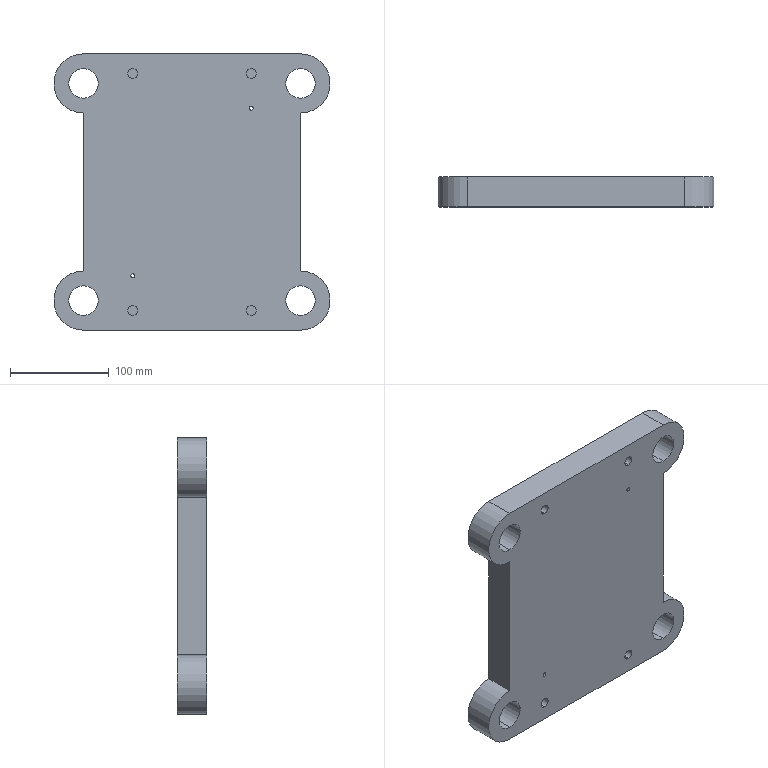Part | SolidWorks | features ICE 4, Extrusion 1, Fillet 1, HoleWzd 1, MirrorPattern 1 | 1 solid | 51 faces | box 280 x 30 x 280 mm | volume 1868516 mm3 | cylinder 34 | plane 15 | torus 2 | commonest cylinder face diameters 10 x8 12 x8 30 x8 4 x4 60 x4 80 x2
STEP:
#1=CARTESIAN_POINT('',(0.,5.,-31.));
#2=VERTEX_POINT('',#1);
#3=CARTESIAN_POINT('',(0.,5.,-19.));
#4=VERTEX_POINT('',#3);
#5=CARTESIAN_POINT('',(0.,5.,-25.));
#6=DIRECTION('',(0.,1.,0.));
#7=DIRECTION('',(0.,0.,1.));
#8=AXIS2_PLACEMENT_3D('',#5,#6,#7);
#9=CIRCLE('',#8,6.);
#10=EDGE_CURVE('',#2,#4,#9,.T.);
#11=ORIENTED_EDGE('',*,*,#10,.F.);
#12=CARTESIAN_POINT('',(0.,20.,-31.));
#13=VERTEX_POINT('',#12);
#14=CARTESIAN_POINT('',(0.,5.,-31.));
#15=DIRECTION('',(0.,1.,0.));
#16=VECTOR('',#15,1000.);
#17=LINE('',#14,#16);
#18=EDGE_CURVE('',#2,#13,#17,.T.);
#19=ORIENTED_EDGE('',*,*,#18,.T.);
#20=CARTESIAN_POINT('',(0.,20.,-19.));
#21=VERTEX_POINT('',#20);
#22=CARTESIAN_POINT('',(0.,20.,-25.));
#23=DIRECTION('',(0.,1.,0.));
#24=DIRECTION('',(0.,0.,1.));
#25=AXIS2_PLACEMENT_3D('',#22,#23,#24);
#26=CIRCLE('',#25,6.);
#27=EDGE_CURVE('',#13,#21,#26,.T.);
#28=ORIENTED_EDGE('',*,*,#27,.T.);
#29=CARTESIAN_POINT('',(0.,5.,-19.));
#30=DIRECTION('',(0.,1.,0.));
#31=VECTOR('',#30,1000.);
#32=LINE('',#29,#31);
#33=EDGE_CURVE('',#4,#21,#32,.T.);
#34=ORIENTED_EDGE('',*,*,#33,.F.);
#35=EDGE_LOOP('',(#11,#19,#28,#34));
#36=FACE_OUTER_BOUND('',#35,.T.);
#37=CARTESIAN_POINT('',(0.,5.,-25.));
#38=DIRECTION('',(0.,1.,0.));
#39=DIRECTION('',(0.,0.,1.));
#40=AXIS2_PLACEMENT_3D('',#37,#38,#39);
#41=CYLINDRICAL_SURFACE('',#40,6.);
#42=ADVANCED_FACE('',(#36),#41,.F.);
#43=CARTESIAN_POINT('',(-25.4,5.,-6.));
#44=VERTEX_POINT('',#43);
#45=CARTESIAN_POINT('',(-25.4,5.,6.));
#46=VERTEX_POINT('',#45);
#47=CARTESIAN_POINT('',(-25.4,5.,0.));
#48=DIRECTION('',(0.,1.,0.));
#49=DIRECTION('',(0.,0.,1.));
#50=AXIS2_PLACEMENT_3D('',#47,#48,#49);
#51=CIRCLE('',#50,6.);
#52=EDGE_CURVE('',#44,#46,#51,.T.);
#53=ORIENTED_EDGE('',*,*,#52,.F.);
#54=CARTESIAN_POINT('',(-25.4,20.,-6.));
#55=VERTEX_POINT('',#54);
#56=CARTESIAN_POINT('',(-25.4,5.,-6.));
#57=DIRECTION('',(0.,1.,0.));
#58=VECTOR('',#57,1000.);
#59=LINE('',#56,#58);
#60=EDGE_CURVE('',#44,#55,#59,.T.);
#61=ORIENTED_EDGE('',*,*,#60,.T.);
#62=CARTESIAN_POINT('',(-25.4,20.,6.));
#63=VERTEX_POINT('',#62);
#64=CARTESIAN_POINT('',(-25.4,20.,0.));
#65=DIRECTION('',(0.,1.,0.));
#66=DIRECTION('',(0.,0.,1.));
#67=AXIS2_PLACEMENT_3D('',#64,#65,#66);
#68=CIRCLE('',#67,6.);
#69=EDGE_CURVE('',#55,#63,#68,.T.);
#70=ORIENTED_EDGE('',*,*,#69,.T.);
#71=CARTESIAN_POINT('',(-25.4,5.,6.));
#72=DIRECTION('',(0.,1.,0.));
#73=VECTOR('',#72,1000.);
#74=LINE('',#71,#73);
#75=EDGE_CURVE('',#46,#63,#74,.T.);
#76=ORIENTED_EDGE('',*,*,#75,.F.);
#77=EDGE_LOOP('',(#53,#61,#70,#76));
#78=FACE_OUTER_BOUND('',#77,.T.);
#79=CARTESIAN_POINT('',(-25.4,5.,0.));
#80=DIRECTION('',(0.,1.,0.));
#81=DIRECTION('',(0.,0.,1.));
#82=AXIS2_PLACEMENT_3D('',#79,#80,#81);
#83=CYLINDRICAL_SURFACE('',#82,6.);
#84=ADVANCED_FACE('',(#78),#83,.F.);
#85=CARTESIAN_POINT('',(0.,5.,19.));
#86=VERTEX_POINT('',#85);
#87=CARTESIAN_POINT('',(0.,5.,31.));
#88=VERTEX_POINT('',#87);
#89=CARTESIAN_POINT('',(0.,5.,25.));
#90=DIRECTION('',(0.,1.,0.));
#91=DIRECTION('',(0.,0.,1.));
#92=AXIS2_PLACEMENT_3D('',#89,#90,#91);
#93=CIRCLE('',#92,6.);
#94=EDGE_CURVE('',#86,#88,#93,.T.);
#95=ORIENTED_EDGE('',*,*,#94,.F.);
#96=CARTESIAN_POINT('',(0.,20.,19.));
#97=VERTEX_POINT('',#96);
#98=CARTESIAN_POINT('',(0.,5.,19.));
#99=DIRECTION('',(0.,1.,0.));
#100=VECTOR('',#99,1000.);
#101=LINE('',#98,#100);
#102=EDGE_CURVE('',#86,#97,#101,.T.);
#103=ORIENTED_EDGE('',*,*,#102,.T.);
#104=CARTESIAN_POINT('',(0.,20.,31.));
#105=VERTEX_POINT('',#104);
#106=CARTESIAN_POINT('',(0.,20.,25.));
#107=DIRECTION('',(0.,1.,0.));
#108=DIRECTION('',(0.,0.,1.));
#109=AXIS2_PLACEMENT_3D('',#106,#107,#108);
#110=CIRCLE('',#109,6.);
#111=EDGE_CURVE('',#97,#105,#110,.T.);
#112=ORIENTED_EDGE('',*,*,#111,.T.);
#113=CARTESIAN_POINT('',(0.,5.,31.));
#114=DIRECTION('',(0.,1.,0.));
#115=VECTOR('',#114,1000.);
#116=LINE('',#113,#115);
#117=EDGE_CURVE('',#88,#105,#116,.T.);
#118=ORIENTED_EDGE('',*,*,#117,.F.);
#119=EDGE_LOOP('',(#95,#103,#112,#118));
#120=FACE_OUTER_BOUND('',#119,.T.);
#121=CARTESIAN_POINT('',(0.,5.,25.));
#122=DIRECTION('',(0.,1.,0.));
#123=DIRECTION('',(0.,0.,1.));
#124=AXIS2_PLACEMENT_3D('',#121,#122,#123);
#125=CYLINDRICAL_SURFACE('',#124,6.);
#126=ADVANCED_FACE('',(#120),#125,.F.);
#127=CARTESIAN_POINT('',(25.,5.,-6.));
#128=VERTEX_POINT('',#127);
#129=CARTESIAN_POINT('',(25.,5.,6.));
#130=VERTEX_POINT('',#129);
#131=CARTESIAN_POINT('',(25.,5.,0.));
#132=DIRECTION('',(0.,1.,0.));
#133=DIRECTION('',(0.,0.,1.));
#134=AXIS2_PLACEMENT_3D('',#131,#132,#133);
#135=CIRCLE('',#134,6.);
#136=EDGE_CURVE('',#128,#130,#135,.T.);
#137=ORIENTED_EDGE('',*,*,#136,.F.);
#138=CARTESIAN_POINT('',(25.,20.,-6.));
#139=VERTEX_POINT('',#138);
#140=CARTESIAN_POINT('',(25.,5.,-6.));
#141=DIRECTION('',(0.,1.,0.));
#142=VECTOR('',#141,1000.);
#143=LINE('',#140,#142);
#144=EDGE_CURVE('',#128,#139,#143,.T.);
#145=ORIENTED_EDGE('',*,*,#144,.T.);
#146=CARTESIAN_POINT('',(25.,20.,6.));
#147=VERTEX_POINT('',#146);
#148=CARTESIAN_POINT('',(25.,20.,0.));
#149=DIRECTION('',(0.,1.,0.));
#150=DIRECTION('',(0.,0.,1.));
#151=AXIS2_PLACEMENT_3D('',#148,#149,#150);
#152=CIRCLE('',#151,6.);
#153=EDGE_CURVE('',#139,#147,#152,.T.);
#154=ORIENTED_EDGE('',*,*,#153,.T.);
#155=CARTESIAN_POINT('',(25.,5.,6.));
#156=DIRECTION('',(0.,1.,0.));
#157=VECTOR('',#156,1000.);
#158=LINE('',#155,#157);
#159=EDGE_CURVE('',#130,#147,#158,.T.);
#160=ORIENTED_EDGE('',*,*,#159,.F.);
#161=EDGE_LOOP('',(#137,#145,#154,#160));
#162=FACE_OUTER_BOUND('',#161,.T.);
#163=CARTESIAN_POINT('',(25.,5.,0.));
#164=DIRECTION('',(0.,1.,0.));
#165=DIRECTION('',(0.,0.,1.));
#166=AXIS2_PLACEMENT_3D('',#163,#164,#165);
#167=CYLINDRICAL_SURFACE('',#166,6.);
#168=ADVANCED_FACE('',(#162),#167,.F.);
#169=CARTESIAN_POINT('',(0.,30.,-42.));
#170=VERTEX_POINT('',#169);
#171=CARTESIAN_POINT('',(0.,30.,42.));
#172=VERTEX_POINT('',#171);
#173=CARTESIAN_POINT('',(0.,30.,0.));
#174=DIRECTION('',(0.,-1.,0.));
#175=DIRECTION('',(0.,0.,1.));
#176=AXIS2_PLACEMENT_3D('',#173,#174,#175);
#177=CIRCLE('',#176,42.);
#178=EDGE_CURVE('',#170,#172,#177,.T.);
#179=ORIENTED_EDGE('',*,*,#178,.F.);
#180=CARTESIAN_POINT('',(0.,28.,-40.));
#181=VERTEX_POINT('',#180);
#182=CARTESIAN_POINT('',(0.,28.,-42.));
#183=DIRECTION('',(1.,0.,0.));
#184=DIRECTION('',(0.,0.,-1.));
#185=AXIS2_PLACEMENT_3D('',#182,#183,#184);
#186=CIRCLE('',#185,2.);
#187=EDGE_CURVE('',#170,#181,#186,.T.);
#188=ORIENTED_EDGE('',*,*,#187,.T.);
#189=CARTESIAN_POINT('',(0.,28.,40.));
#190=VERTEX_POINT('',#189);
#191=CARTESIAN_POINT('',(0.,28.,0.));
#192=DIRECTION('',(0.,1.,0.));
#193=DIRECTION('',(0.,0.,1.));
#194=AXIS2_PLACEMENT_3D('',#191,#192,#193);
#195=CIRCLE('',#194,40.);
#196=EDGE_CURVE('',#190,#181,#195,.T.);
#197=ORIENTED_EDGE('',*,*,#196,.F.);
#198=CARTESIAN_POINT('',(0.,28.,42.));
#199=DIRECTION('',(-1.,0.,0.));
#200=DIRECTION('',(0.,0.,1.));
#201=AXIS2_PLACEMENT_3D('',#198,#199,#200);
#202=CIRCLE('',#201,2.);
#203=EDGE_CURVE('',#172,#190,#202,.T.);
#204=ORIENTED_EDGE('',*,*,#203,.F.);
#205=EDGE_LOOP('',(#179,#188,#197,#204));
#206=FACE_OUTER_BOUND('',#205,.T.);
#207=CARTESIAN_POINT('',(0.,28.,0.));
#208=DIRECTION('',(0.,1.,0.));
#209=DIRECTION('',(0.,0.,1.));
#210=AXIS2_PLACEMENT_3D('',#207,#208,#209);
#211=TOROIDAL_SURFACE('',#210,42.,2.);
#212=ADVANCED_FACE('',(#206),#211,.T.);
#213=CARTESIAN_POINT('',(0.,20.,-40.));
#214=VERTEX_POINT('',#213);
#215=CARTESIAN_POINT('',(0.,20.,40.));
#216=VERTEX_POINT('',#215);
#217=CARTESIAN_POINT('',(0.,20.,0.));
#218=DIRECTION('',(0.,1.,0.));
#219=DIRECTION('',(0.,0.,1.));
#220=AXIS2_PLACEMENT_3D('',#217,#218,#219);
#221=CIRCLE('',#220,40.);
#222=EDGE_CURVE('',#214,#216,#221,.T.);
#223=ORIENTED_EDGE('',*,*,#222,.F.);
#224=CARTESIAN_POINT('',(0.,20.,-40.));
#225=DIRECTION('',(0.,1.,0.));
#226=VECTOR('',#225,1000.);
#227=LINE('',#224,#226);
#228=EDGE_CURVE('',#214,#181,#227,.T.);
#229=ORIENTED_EDGE('',*,*,#228,.T.);
#230=CARTESIAN_POINT('',(0.,28.,0.));
#231=DIRECTION('',(0.,1.,0.));
#232=DIRECTION('',(0.,0.,1.));
#233=AXIS2_PLACEMENT_3D('',#230,#231,#232);
#234=CIRCLE('',#233,40.);
#235=EDGE_CURVE('',#181,#190,#234,.T.);
#236=ORIENTED_EDGE('',*,*,#235,.T.);
#237=CARTESIAN_POINT('',(0.,20.,40.));
#238=DIRECTION('',(0.,1.,0.));
#239=VECTOR('',#238,1000.);
#240=LINE('',#237,#239);
#241=EDGE_CURVE('',#216,#190,#240,.T.);
#242=ORIENTED_EDGE('',*,*,#241,.F.);
#243=EDGE_LOOP('',(#223,#229,#236,#242));
#244=FACE_OUTER_BOUND('',#243,.T.);
#245=CARTESIAN_POINT('',(0.,20.,0.));
#246=DIRECTION('',(0.,1.,0.));
#247=DIRECTION('',(0.,0.,1.));
#248=AXIS2_PLACEMENT_3D('',#245,#246,#247);
#249=CYLINDRICAL_SURFACE('',#248,40.);
#250=ADVANCED_FACE('',(#244),#249,.F.);
#251=CARTESIAN_POINT('',(-60.,20.,-115.));
#252=VERTEX_POINT('',#251);
#253=CARTESIAN_POINT('',(-60.,20.,-125.));
#254=VERTEX_POINT('',#253);
#255=CARTESIAN_POINT('',(-60.,20.,-120.));
#256=DIRECTION('',(0.,-1.,0.));
#257=DIRECTION('',(0.,0.,1.));
#258=AXIS2_PLACEMENT_3D('',#255,#256,#257);
#259=CIRCLE('',#258,5.);
#260=EDGE_CURVE('',#252,#254,#259,.T.);
#261=ORIENTED_EDGE('',*,*,#260,.F.);
#262=CARTESIAN_POINT('',(-60.,0.,-115.));
#263=VERTEX_POINT('',#262);
#264=CARTESIAN_POINT('',(-60.,20.,-115.));
#265=DIRECTION('',(0.,-1.,0.));
#266=VECTOR('',#265,1000.);
#267=LINE('',#264,#266);
#268=EDGE_CURVE('',#252,#263,#267,.T.);
#269=ORIENTED_EDGE('',*,*,#268,.T.);
#270=CARTESIAN_POINT('',(-60.,0.,-125.));
#271=VERTEX_POINT('',#270);
#272=CARTESIAN_POINT('',(-60.,0.,-120.));
#273=DIRECTION('',(0.,-1.,0.));
#274=DIRECTION('',(0.,0.,1.));
#275=AXIS2_PLACEMENT_3D('',#272,#273,#274);
#276=CIRCLE('',#275,5.);
#277=EDGE_CURVE('',#263,#271,#276,.T.);
#278=ORIENTED_EDGE('',*,*,#277,.T.);
#279=CARTESIAN_POINT('',(-60.,20.,-125.));
#280=DIRECTION('',(0.,-1.,0.));
#281=VECTOR('',#280,1000.);
#282=LINE('',#279,#281);
#283=EDGE_CURVE('',#254,#271,#282,.T.);
#284=ORIENTED_EDGE('',*,*,#283,.F.);
#285=EDGE_LOOP('',(#261,#269,#278,#284));
#286=FACE_OUTER_BOUND('',#285,.T.);
#287=CARTESIAN_POINT('',(-60.,20.,-120.));
#288=DIRECTION('',(0.,-1.,0.));
#289=DIRECTION('',(0.,0.,-1.));
#290=AXIS2_PLACEMENT_3D('',#287,#288,#289);
#291=CYLINDRICAL_SURFACE('',#290,5.);
#292=ADVANCED_FACE('',(#286),#291,.F.);
#293=CARTESIAN_POINT('',(60.,20.,-115.));
#294=VERTEX_POINT('',#293);
#295=CARTESIAN_POINT('',(60.,20.,-125.));
#296=VERTEX_POINT('',#295);
#297=CARTESIAN_POINT('',(60.,20.,-120.));
#298=DIRECTION('',(0.,-1.,0.));
#299=DIRECTION('',(0.,0.,-1.));
#300=AXIS2_PLACEMENT_3D('',#297,#298,#299);
#301=CIRCLE('',#300,5.);
#302=EDGE_CURVE('',#294,#296,#301,.T.);
#303=ORIENTED_EDGE('',*,*,#302,.F.);
#304=CARTESIAN_POINT('',(60.,0.,-115.));
#305=VERTEX_POINT('',#304);
#306=CARTESIAN_POINT('',(60.,20.,-115.));
#307=DIRECTION('',(0.,-1.,0.));
#308=VECTOR('',#307,1000.);
#309=LINE('',#306,#308);
#310=EDGE_CURVE('',#294,#305,#309,.T.);
#311=ORIENTED_EDGE('',*,*,#310,.T.);
#312=CARTESIAN_POINT('',(60.,0.,-125.));
#313=VERTEX_POINT('',#312);
#314=CARTESIAN_POINT('',(60.,0.,-120.));
#315=DIRECTION('',(0.,-1.,0.));
#316=DIRECTION('',(0.,0.,-1.));
#317=AXIS2_PLACEMENT_3D('',#314,#315,#316);
#318=CIRCLE('',#317,5.);
#319=EDGE_CURVE('',#305,#313,#318,.T.);
#320=ORIENTED_EDGE('',*,*,#319,.T.);
#321=CARTESIAN_POINT('',(60.,20.,-125.));
#322=DIRECTION('',(0.,-1.,0.));
#323=VECTOR('',#322,1000.);
#324=LINE('',#321,#323);
#325=EDGE_CURVE('',#296,#313,#324,.T.);
#326=ORIENTED_EDGE('',*,*,#325,.F.);
#327=EDGE_LOOP('',(#303,#311,#320,#326));
#328=FACE_OUTER_BOUND('',#327,.T.);
#329=CARTESIAN_POINT('',(60.,20.,-120.));
#330=DIRECTION('',(0.,-1.,0.));
#331=DIRECTION('',(0.,0.,-1.));
#332=AXIS2_PLACEMENT_3D('',#329,#330,#331);
#333=CYLINDRICAL_SURFACE('',#332,5.);
#334=ADVANCED_FACE('',(#328),#333,.F.);
#335=CARTESIAN_POINT('',(60.,20.,125.));
#336=VERTEX_POINT('',#335);
#337=CARTESIAN_POINT('',(60.,20.,115.));
#338=VERTEX_POINT('',#337);
#339=CARTESIAN_POINT('',(60.,20.,120.));
#340=DIRECTION('',(0.,-1.,0.));
#341=DIRECTION('',(0.,0.,1.));
#342=AXIS2_PLACEMENT_3D('',#339,#340,#341);
#343=CIRCLE('',#342,5.);
#344=EDGE_CURVE('',#336,#338,#343,.T.);
#345=ORIENTED_EDGE('',*,*,#344,.F.);
#346=CARTESIAN_POINT('',(60.,0.,125.));
#347=VERTEX_POINT('',#346);
#348=CARTESIAN_POINT('',(60.,20.,125.));
#349=DIRECTION('',(0.,-1.,0.));
#350=VECTOR('',#349,1000.);
#351=LINE('',#348,#350);
#352=EDGE_CURVE('',#336,#347,#351,.T.);
#353=ORIENTED_EDGE('',*,*,#352,.T.);
#354=CARTESIAN_POINT('',(60.,0.,115.));
#355=VERTEX_POINT('',#354);
#356=CARTESIAN_POINT('',(60.,0.,120.));
#357=DIRECTION('',(0.,-1.,0.));
#358=DIRECTION('',(0.,0.,1.));
#359=AXIS2_PLACEMENT_3D('',#356,#357,#358);
#360=CIRCLE('',#359,5.);
#361=EDGE_CURVE('',#347,#355,#360,.T.);
#362=ORIENTED_EDGE('',*,*,#361,.T.);
#363=CARTESIAN_POINT('',(60.,20.,115.));
#364=DIRECTION('',(0.,-1.,0.));
#365=VECTOR('',#364,1000.);
#366=LINE('',#363,#365);
#367=EDGE_CURVE('',#338,#355,#366,.T.);
#368=ORIENTED_EDGE('',*,*,#367,.F.);
#369=EDGE_LOOP('',(#345,#353,#362,#368));
#370=FACE_OUTER_BOUND('',#369,.T.);
#371=CARTESIAN_POINT('',(60.,20.,120.));
#372=DIRECTION('',(0.,-1.,0.));
#373=DIRECTION('',(0.,0.,-1.));
#374=AXIS2_PLACEMENT_3D('',#371,#372,#373);
#375=CYLINDRICAL_SURFACE('',#374,5.);
#376=ADVANCED_FACE('',(#370),#375,.F.);
#377=CARTESIAN_POINT('',(-60.,20.,125.));
#378=VERTEX_POINT('',#377);
#379=CARTESIAN_POINT('',(-60.,20.,115.));
#380=VERTEX_POINT('',#379);
#381=CARTESIAN_POINT('',(-60.,20.,120.));
#382=DIRECTION('',(0.,-1.,0.));
#383=DIRECTION('',(0.,0.,-1.));
#384=AXIS2_PLACEMENT_3D('',#381,#382,#383);
#385=CIRCLE('',#384,5.);
#386=EDGE_CURVE('',#378,#380,#385,.T.);
#387=ORIENTED_EDGE('',*,*,#386,.F.);
#388=CARTESIAN_POINT('',(-60.,0.,125.));
#389=VERTEX_POINT('',#388);
#390=CARTESIAN_POINT('',(-60.,20.,125.));
#391=DIRECTION('',(0.,-1.,0.));
#392=VECTOR('',#391,1000.);
#393=LINE('',#390,#392);
#394=EDGE_CURVE('',#378,#389,#393,.T.);
#395=ORIENTED_EDGE('',*,*,#394,.T.);
#396=CARTESIAN_POINT('',(-60.,0.,115.));
#397=VERTEX_POINT('',#396);
#398=CARTESIAN_POINT('',(-60.,0.,120.));
#399=DIRECTION('',(0.,-1.,0.));
#400=DIRECTION('',(0.,0.,-1.));
#401=AXIS2_PLACEMENT_3D('',#398,#399,#400);
#402=CIRCLE('',#401,5.);
#403=EDGE_CURVE('',#389,#397,#402,.T.);
#404=ORIENTED_EDGE('',*,*,#403,.T.);
#405=CARTESIAN_POINT('',(-60.,20.,115.));
#406=DIRECTION('',(0.,-1.,0.));
#407=VECTOR('',#406,1000.);
#408=LINE('',#405,#407);
#409=EDGE_CURVE('',#380,#397,#408,.T.);
#410=ORIENTED_EDGE('',*,*,#409,.F.);
#411=EDGE_LOOP('',(#387,#395,#404,#410));
#412=FACE_OUTER_BOUND('',#411,.T.);
#413=CARTESIAN_POINT('',(-60.,20.,120.));
#414=DIRECTION('',(0.,-1.,0.));
#415=DIRECTION('',(0.,0.,-1.));
#416=AXIS2_PLACEMENT_3D('',#413,#414,#415);
#417=CYLINDRICAL_SURFACE('',#416,5.);
#418=ADVANCED_FACE('',(#412),#417,.F.);
#419=CARTESIAN_POINT('',(-60.,0.,-87.));
#420=VERTEX_POINT('',#419);
#421=CARTESIAN_POINT('',(-60.,0.,-83.));
#422=VERTEX_POINT('',#421);
#423=CARTESIAN_POINT('',(-60.,0.,-85.));
#424=DIRECTION('',(0.,1.,0.));
#425=DIRECTION('',(0.,0.,1.));
#426=AXIS2_PLACEMENT_3D('',#423,#424,#425);
#427=CIRCLE('',#426,2.);
#428=EDGE_CURVE('',#420,#422,#427,.T.);
#429=ORIENTED_EDGE('',*,*,#428,.F.);
#430=CARTESIAN_POINT('',(-60.,30.,-87.));
#431=VERTEX_POINT('',#430);
#432=CARTESIAN_POINT('',(-60.,0.,-87.));
#433=DIRECTION('',(0.,1.,0.));
#434=VECTOR('',#433,1000.);
#435=LINE('',#432,#434);
#436=EDGE_CURVE('',#420,#431,#435,.T.);
#437=ORIENTED_EDGE('',*,*,#436,.T.);
#438=CARTESIAN_POINT('',(-60.,30.,-83.));
#439=VERTEX_POINT('',#438);
#440=CARTESIAN_POINT('',(-60.,30.,-85.));
#441=DIRECTION('',(0.,1.,0.));
#442=DIRECTION('',(0.,0.,1.));
#443=AXIS2_PLACEMENT_3D('',#440,#441,#442);
#444=CIRCLE('',#443,2.);
#445=EDGE_CURVE('',#431,#439,#444,.T.);
#446=ORIENTED_EDGE('',*,*,#445,.T.);
#447=CARTESIAN_POINT('',(-60.,0.,-83.));
#448=DIRECTION('',(0.,1.,0.));
#449=VECTOR('',#448,1000.);
#450=LINE('',#447,#449);
#451=EDGE_CURVE('',#422,#439,#450,.T.);
#452=ORIENTED_EDGE('',*,*,#451,.F.);
#453=EDGE_LOOP('',(#429,#437,#446,#452));
#454=FACE_OUTER_BOUND('',#453,.T.);
#455=CARTESIAN_POINT('',(-60.,0.,-85.));
#456=DIRECTION('',(0.,1.,0.));
#457=DIRECTION('',(0.,0.,1.));
#458=AXIS2_PLACEMENT_3D('',#455,#456,#457);
#459=CYLINDRICAL_SURFACE('',#458,2.);
#460=ADVANCED_FACE('',(#454),#459,.F.);
#461=CARTESIAN_POINT('',(60.,0.,83.));
#462=VERTEX_POINT('',#461);
#463=CARTESIAN_POINT('',(60.,0.,87.));
#464=VERTEX_POINT('',#463);
#465=CARTESIAN_POINT('',(60.,0.,85.));
#466=DIRECTION('',(0.,1.,0.));
#467=DIRECTION('',(0.,0.,1.));
#468=AXIS2_PLACEMENT_3D('',#465,#466,#467);
#469=CIRCLE('',#468,2.);
#470=EDGE_CURVE('',#462,#464,#469,.T.);
#471=ORIENTED_EDGE('',*,*,#470,.F.);
#472=CARTESIAN_POINT('',(60.,30.,83.));
#473=VERTEX_POINT('',#472);
#474=CARTESIAN_POINT('',(60.,0.,83.));
#475=DIRECTION('',(0.,1.,0.));
#476=VECTOR('',#475,1000.);
#477=LINE('',#474,#476);
#478=EDGE_CURVE('',#462,#473,#477,.T.);
#479=ORIENTED_EDGE('',*,*,#478,.T.);
#480=CARTESIAN_POINT('',(60.,30.,87.));
#481=VERTEX_POINT('',#480);
#482=CARTESIAN_POINT('',(60.,30.,85.));
#483=DIRECTION('',(0.,1.,0.));
#484=DIRECTION('',(0.,0.,1.));
#485=AXIS2_PLACEMENT_3D('',#482,#483,#484);
#486=CIRCLE('',#485,2.);
#487=EDGE_CURVE('',#473,#481,#486,.T.);
#488=ORIENTED_EDGE('',*,*,#487,.T.);
#489=CARTESIAN_POINT('',(60.,0.,87.));
#490=DIRECTION('',(0.,1.,0.));
#491=VECTOR('',#490,1000.);
#492=LINE('',#489,#491);
#493=EDGE_CURVE('',#464,#481,#492,.T.);
#494=ORIENTED_EDGE('',*,*,#493,.F.);
#495=EDGE_LOOP('',(#471,#479,#488,#494));
#496=FACE_OUTER_BOUND('',#495,.T.);
#497=CARTESIAN_POINT('',(60.,0.,85.));
#498=DIRECTION('',(0.,1.,0.));
#499=DIRECTION('',(0.,0.,1.));
#500=AXIS2_PLACEMENT_3D('',#497,#498,#499);
#501=CYLINDRICAL_SURFACE('',#500,2.);
#502=ADVANCED_FACE('',(#496),#501,.F.);
#503=CARTESIAN_POINT('',(110.,30.,125.));
#504=VERTEX_POINT('',#503);
#505=CARTESIAN_POINT('',(110.,30.,95.));
#506=VERTEX_POINT('',#505);
#507=CARTESIAN_POINT('',(110.,30.,110.));
#508=DIRECTION('',(0.,-1.,0.));
#509=DIRECTION('',(0.,0.,1.));
#510=AXIS2_PLACEMENT_3D('',#507,#508,#509);
#511=CIRCLE('',#510,15.);
#512=EDGE_CURVE('',#504,#506,#511,.T.);
#513=ORIENTED_EDGE('',*,*,#512,.F.);
#514=CARTESIAN_POINT('',(110.,0.,125.));
#515=VERTEX_POINT('',#514);
#516=CARTESIAN_POINT('',(110.,30.,125.));
#517=DIRECTION('',(0.,-1.,0.));
#518=VECTOR('',#517,1000.);
#519=LINE('',#516,#518);
#520=EDGE_CURVE('',#504,#515,#519,.T.);
#521=ORIENTED_EDGE('',*,*,#520,.T.);
#522=CARTESIAN_POINT('',(110.,0.,95.));
#523=VERTEX_POINT('',#522);
#524=CARTESIAN_POINT('',(110.,0.,110.));
#525=DIRECTION('',(0.,-1.,0.));
#526=DIRECTION('',(0.,0.,1.));
#527=AXIS2_PLACEMENT_3D('',#524,#525,#526);
#528=CIRCLE('',#527,15.);
#529=EDGE_CURVE('',#515,#523,#528,.T.);
#530=ORIENTED_EDGE('',*,*,#529,.T.);
#531=CARTESIAN_POINT('',(110.,30.,95.));
#532=DIRECTION('',(0.,-1.,0.));
#533=VECTOR('',#532,1000.);
#534=LINE('',#531,#533);
#535=EDGE_CURVE('',#506,#523,#534,.T.);
#536=ORIENTED_EDGE('',*,*,#535,.F.);
#537=EDGE_LOOP('',(#513,#521,#530,#536));
#538=FACE_OUTER_BOUND('',#537,.T.);
#539=CARTESIAN_POINT('',(110.,30.,110.));
#540=DIRECTION('',(0.,-1.,0.));
#541=DIRECTION('',(0.,0.,-1.));
#542=AXIS2_PLACEMENT_3D('',#539,#540,#541);
#543=CYLINDRICAL_SURFACE('',#542,15.);
#544=ADVANCED_FACE('',(#538),#543,.F.);
#545=CARTESIAN_POINT('',(110.,30.,-95.));
#546=VERTEX_POINT('',#545);
#547=CARTESIAN_POINT('',(110.,30.,-125.));
#548=VERTEX_POINT('',#547);
#549=CARTESIAN_POINT('',(110.,30.,-110.));
#550=DIRECTION('',(0.,-1.,0.));
#551=DIRECTION('',(0.,0.,1.));
#552=AXIS2_PLACEMENT_3D('',#549,#550,#551);
#553=CIRCLE('',#552,15.);
#554=EDGE_CURVE('',#546,#548,#553,.T.);
#555=ORIENTED_EDGE('',*,*,#554,.F.);
#556=CARTESIAN_POINT('',(110.,0.,-95.));
#557=VERTEX_POINT('',#556);
#558=CARTESIAN_POINT('',(110.,30.,-95.));
#559=DIRECTION('',(0.,-1.,0.));
#560=VECTOR('',#559,1000.);
#561=LINE('',#558,#560);
#562=EDGE_CURVE('',#546,#557,#561,.T.);
#563=ORIENTED_EDGE('',*,*,#562,.T.);
#564=CARTESIAN_POINT('',(110.,0.,-125.));
#565=VERTEX_POINT('',#564);
#566=CARTESIAN_POINT('',(110.,0.,-110.));
#567=DIRECTION('',(0.,-1.,0.));
#568=DIRECTION('',(0.,0.,1.));
#569=AXIS2_PLACEMENT_3D('',#566,#567,#568);
#570=CIRCLE('',#569,15.);
#571=EDGE_CURVE('',#557,#565,#570,.T.);
#572=ORIENTED_EDGE('',*,*,#571,.T.);
#573=CARTESIAN_POINT('',(110.,30.,-125.));
#574=DIRECTION('',(0.,-1.,0.));
#575=VECTOR('',#574,1000.);
#576=LINE('',#573,#575);
#577=EDGE_CURVE('',#548,#565,#576,.T.);
#578=ORIENTED_EDGE('',*,*,#577,.F.);
#579=EDGE_LOOP('',(#555,#563,#572,#578));
#580=FACE_OUTER_BOUND('',#579,.T.);
#581=CARTESIAN_POINT('',(110.,30.,-110.));
#582=DIRECTION('',(0.,-1.,0.));
#583=DIRECTION('',(0.,0.,-1.));
#584=AXIS2_PLACEMENT_3D('',#581,#582,#583);
#585=CYLINDRICAL_SURFACE('',#584,15.);
#586=ADVANCED_FACE('',(#580),#585,.F.);
#587=CARTESIAN_POINT('',(-110.,30.,95.));
#588=VERTEX_POINT('',#587);
#589=CARTESIAN_POINT('',(-110.,30.,125.));
#590=VERTEX_POINT('',#589);
#591=CARTESIAN_POINT('',(-110.,30.,110.));
#592=DIRECTION('',(0.,1.,0.));
#593=DIRECTION('',(0.,0.,1.));
#594=AXIS2_PLACEMENT_3D('',#591,#592,#593);
#595=CIRCLE('',#594,15.);
#596=EDGE_CURVE('',#588,#590,#595,.T.);
#597=ORIENTED_EDGE('',*,*,#596,.T.);
#598=CARTESIAN_POINT('',(-110.,0.,125.));
#599=VERTEX_POINT('',#598);
#600=CARTESIAN_POINT('',(-110.,30.,125.));
#601=DIRECTION('',(0.,-1.,0.));
#602=VECTOR('',#601,1000.);
#603=LINE('',#600,#602);
#604=EDGE_CURVE('',#590,#599,#603,.T.);
#605=ORIENTED_EDGE('',*,*,#604,.T.);
#606=CARTESIAN_POINT('',(-110.,0.,95.));
#607=VERTEX_POINT('',#606);
#608=CARTESIAN_POINT('',(-110.,0.,110.));
#609=DIRECTION('',(0.,1.,0.));
#610=DIRECTION('',(0.,0.,1.));
#611=AXIS2_PLACEMENT_3D('',#608,#609,#610);
#612=CIRCLE('',#611,15.);
#613=EDGE_CURVE('',#607,#599,#612,.T.);
#614=ORIENTED_EDGE('',*,*,#613,.F.);
#615=CARTESIAN_POINT('',(-110.,30.,95.));
#616=DIRECTION('',(0.,-1.,0.));
#617=VECTOR('',#616,1000.);
#618=LINE('',#615,#617);
#619=EDGE_CURVE('',#588,#607,#618,.T.);
#620=ORIENTED_EDGE('',*,*,#619,.F.);
#621=EDGE_LOOP('',(#597,#605,#614,#620));
#622=FACE_OUTER_BOUND('',#621,.T.);
#623=CARTESIAN_POINT('',(-110.,30.,110.));
#624=DIRECTION('',(0.,-1.,0.));
#625=DIRECTION('',(0.,0.,-1.));
#626=AXIS2_PLACEMENT_3D('',#623,#624,#625);
#627=CYLINDRICAL_SURFACE('',#626,15.);
#628=ADVANCED_FACE('',(#622),#627,.F.);
#629=CARTESIAN_POINT('',(-110.,30.,-125.));
#630=VERTEX_POINT('',#629);
#631=CARTESIAN_POINT('',(-110.,30.,-95.));
#632=VERTEX_POINT('',#631);
#633=CARTESIAN_POINT('',(-110.,30.,-110.));
#634=DIRECTION('',(0.,1.,0.));
#635=DIRECTION('',(0.,0.,1.));
#636=AXIS2_PLACEMENT_3D('',#633,#634,#635);
#637=CIRCLE('',#636,15.);
#638=EDGE_CURVE('',#630,#632,#637,.T.);
#639=ORIENTED_EDGE('',*,*,#638,.T.);
#640=CARTESIAN_POINT('',(-110.,0.,-95.));
#641=VERTEX_POINT('',#640);
#642=CARTESIAN_POINT('',(-110.,30.,-95.));
#643=DIRECTION('',(0.,-1.,0.));
#644=VECTOR('',#643,1000.);
#645=LINE('',#642,#644);
#646=EDGE_CURVE('',#632,#641,#645,.T.);
#647=ORIENTED_EDGE('',*,*,#646,.T.);
#648=CARTESIAN_POINT('',(-110.,0.,-125.));
#649=VERTEX_POINT('',#648);
#650=CARTESIAN_POINT('',(-110.,0.,-110.));
#651=DIRECTION('',(0.,1.,0.));
#652=DIRECTION('',(0.,0.,1.));
#653=AXIS2_PLACEMENT_3D('',#650,#651,#652);
#654=CIRCLE('',#653,15.);
#655=EDGE_CURVE('',#649,#641,#654,.T.);
#656=ORIENTED_EDGE('',*,*,#655,.F.);
#657=CARTESIAN_POINT('',(-110.,30.,-125.));
#658=DIRECTION('',(0.,-1.,0.));
#659=VECTOR('',#658,1000.);
#660=LINE('',#657,#659);
#661=EDGE_CURVE('',#630,#649,#660,.T.);
#662=ORIENTED_EDGE('',*,*,#661,.F.);
#663=EDGE_LOOP('',(#639,#647,#656,#662));
#664=FACE_OUTER_BOUND('',#663,.T.);
#665=CARTESIAN_POINT('',(-110.,30.,-110.));
#666=DIRECTION('',(0.,-1.,0.));
#667=DIRECTION('',(0.,0.,-1.));
#668=AXIS2_PLACEMENT_3D('',#665,#666,#667);
#669=CYLINDRICAL_SURFACE('',#668,15.);
#670=ADVANCED_FACE('',(#664),#669,.F.);
#671=CARTESIAN_POINT('',(0.,30.,0.));
#672=DIRECTION('',(0.,-1.,0.));
#673=DIRECTION('',(0.,0.,1.));
#674=AXIS2_PLACEMENT_3D('',#671,#672,#673);
#675=CIRCLE('',#674,42.);
#676=EDGE_CURVE('',#172,#170,#675,.T.);
#677=ORIENTED_EDGE('',*,*,#676,.T.);
#678=ORIENTED_EDGE('',*,*,#178,.T.);
#679=EDGE_LOOP('',(#677,#678));
#680=FACE_BOUND('',#679,.T.);
#681=CARTESIAN_POINT('',(-60.,30.,-85.));
#682=DIRECTION('',(0.,1.,0.));
#683=DIRECTION('',(0.,0.,1.));
#684=AXIS2_PLACEMENT_3D('',#681,#682,#683);
#685=CIRCLE('',#684,2.);
#686=EDGE_CURVE('',#439,#431,#685,.T.);
#687=ORIENTED_EDGE('',*,*,#686,.F.);
#688=ORIENTED_EDGE('',*,*,#445,.F.);
#689=EDGE_LOOP('',(#687,#688));
#690=FACE_BOUND('',#689,.T.);
#691=CARTESIAN_POINT('',(60.,30.,85.));
#692=DIRECTION('',(0.,1.,0.));
#693=DIRECTION('',(0.,0.,1.));
#694=AXIS2_PLACEMENT_3D('',#691,#692,#693);
#695=CIRCLE('',#694,2.);
#696=EDGE_CURVE('',#481,#473,#695,.T.);
#697=ORIENTED_EDGE('',*,*,#696,.F.);
#698=ORIENTED_EDGE('',*,*,#487,.F.);
#699=EDGE_LOOP('',(#697,#698));
#700=FACE_BOUND('',#699,.T.);
#701=CARTESIAN_POINT('',(-110.,30.,140.));
#702=VERTEX_POINT('',#701);
#703=CARTESIAN_POINT('',(110.,30.,140.));
#704=VERTEX_POINT('',#703);
#705=CARTESIAN_POINT('',(-110.,30.,140.));
#706=DIRECTION('',(1.,0.,0.));
#707=VECTOR('',#706,1000.);
#708=LINE('',#705,#707);
#709=EDGE_CURVE('',#702,#704,#708,.T.);
#710=ORIENTED_EDGE('',*,*,#709,.T.);
#711=CARTESIAN_POINT('',(110.,30.,80.));
#712=VERTEX_POINT('',#711);
#713=CARTESIAN_POINT('',(110.,30.,110.));
#714=DIRECTION('',(0.,-1.,0.));
#715=DIRECTION('',(0.,0.,1.));
#716=AXIS2_PLACEMENT_3D('',#713,#714,#715);
#717=CIRCLE('',#716,30.);
#718=EDGE_CURVE('',#712,#704,#717,.T.);
#719=ORIENTED_EDGE('',*,*,#718,.F.);
#720=CARTESIAN_POINT('',(110.,30.,-80.));
#721=VERTEX_POINT('',#720);
#722=CARTESIAN_POINT('',(110.,30.,80.));
#723=DIRECTION('',(0.,0.,1.));
#724=VECTOR('',#723,1000.);
#725=LINE('',#722,#724);
#726=EDGE_CURVE('',#721,#712,#725,.T.);
#727=ORIENTED_EDGE('',*,*,#726,.F.);
#728=CARTESIAN_POINT('',(110.,30.,-140.));
#729=VERTEX_POINT('',#728);
#730=CARTESIAN_POINT('',(110.,30.,-110.));
#731=DIRECTION('',(0.,-1.,0.));
#732=DIRECTION('',(0.,0.,1.));
#733=AXIS2_PLACEMENT_3D('',#730,#731,#732);
#734=CIRCLE('',#733,30.);
#735=EDGE_CURVE('',#729,#721,#734,.T.);
#736=ORIENTED_EDGE('',*,*,#735,.F.);
#737=CARTESIAN_POINT('',(-110.,30.,-140.));
#738=VERTEX_POINT('',#737);
#739=CARTESIAN_POINT('',(80.,30.,-140.));
#740=DIRECTION('',(-1.,0.,0.));
#741=VECTOR('',#740,1000.);
#742=LINE('',#739,#741);
#743=EDGE_CURVE('',#729,#738,#742,.T.);
#744=ORIENTED_EDGE('',*,*,#743,.T.);
#745=CARTESIAN_POINT('',(-110.,30.,-80.));
#746=VERTEX_POINT('',#745);
#747=CARTESIAN_POINT('',(-110.,30.,-110.));
#748=DIRECTION('',(0.,1.,0.));
#749=DIRECTION('',(0.,0.,1.));
#750=AXIS2_PLACEMENT_3D('',#747,#748,#749);
#751=CIRCLE('',#750,30.);
#752=EDGE_CURVE('',#738,#746,#751,.T.);
#753=ORIENTED_EDGE('',*,*,#752,.T.);
#754=CARTESIAN_POINT('',(-110.,30.,80.));
#755=VERTEX_POINT('',#754);
#756=CARTESIAN_POINT('',(-110.,30.,80.));
#757=DIRECTION('',(0.,0.,1.));
#758=VECTOR('',#757,1000.);
#759=LINE('',#756,#758);
#760=EDGE_CURVE('',#746,#755,#759,.T.);
#761=ORIENTED_EDGE('',*,*,#760,.T.);
#762=CARTESIAN_POINT('',(-110.,30.,110.));
#763=DIRECTION('',(0.,1.,0.));
#764=DIRECTION('',(0.,0.,1.));
#765=AXIS2_PLACEMENT_3D('',#762,#763,#764);
#766=CIRCLE('',#765,30.);
#767=EDGE_CURVE('',#755,#702,#766,.T.);
#768=ORIENTED_EDGE('',*,*,#767,.T.);
#769=EDGE_LOOP('',(#710,#719,#727,#736,#744,#753,#761,#768));
#770=FACE_OUTER_BOUND('',#769,.T.);
#771=ORIENTED_EDGE('',*,*,#638,.F.);
#772=CARTESIAN_POINT('',(-110.,30.,-110.));
#773=DIRECTION('',(0.,1.,0.));
#774=DIRECTION('',(0.,0.,1.));
#775=AXIS2_PLACEMENT_3D('',#772,#773,#774);
#776=CIRCLE('',#775,15.);
#777=EDGE_CURVE('',#632,#630,#776,.T.);
#778=ORIENTED_EDGE('',*,*,#777,.F.);
#779=EDGE_LOOP('',(#771,#778));
#780=FACE_BOUND('',#779,.T.);
#781=ORIENTED_EDGE('',*,*,#596,.F.);
#782=CARTESIAN_POINT('',(-110.,30.,110.));
#783=DIRECTION('',(0.,1.,0.));
#784=DIRECTION('',(0.,0.,1.));
#785=AXIS2_PLACEMENT_3D('',#782,#783,#784);
#786=CIRCLE('',#785,15.);
#787=EDGE_CURVE('',#590,#588,#786,.T.);
#788=ORIENTED_EDGE('',*,*,#787,.F.);
#789=EDGE_LOOP('',(#781,#788));
#790=FACE_BOUND('',#789,.T.);
#791=CARTESIAN_POINT('',(110.,30.,-110.));
#792=DIRECTION('',(0.,-1.,0.));
#793=DIRECTION('',(0.,0.,1.));
#794=AXIS2_PLACEMENT_3D('',#791,#792,#793);
#795=CIRCLE('',#794,15.);
#796=EDGE_CURVE('',#548,#546,#795,.T.);
#797=ORIENTED_EDGE('',*,*,#796,.T.);
#798=ORIENTED_EDGE('',*,*,#554,.T.);
#799=EDGE_LOOP('',(#797,#798));
#800=FACE_BOUND('',#799,.T.);
#801=CARTESIAN_POINT('',(110.,30.,110.));
#802=DIRECTION('',(0.,-1.,0.));
#803=DIRECTION('',(0.,0.,1.));
#804=AXIS2_PLACEMENT_3D('',#801,#802,#803);
#805=CIRCLE('',#804,15.);
#806=EDGE_CURVE('',#506,#504,#805,.T.);
#807=ORIENTED_EDGE('',*,*,#806,.T.);
#808=ORIENTED_EDGE('',*,*,#512,.T.);
#809=EDGE_LOOP('',(#807,#808));
#810=FACE_BOUND('',#809,.T.);
#811=CARTESIAN_POINT('',(-110.,30.,-110.));
#812=DIRECTION('',(0.,1.,0.));
#813=DIRECTION('',(0.,0.,1.));
#814=AXIS2_PLACEMENT_3D('',#811,#812,#813);
#815=PLANE('',#814);
#816=ADVANCED_FACE('',(#680,#690,#700,#770,#780,#790,#800,#810),#815,.T.);
#817=CARTESIAN_POINT('',(-60.,0.,-120.));
#818=DIRECTION('',(0.,-1.,0.));
#819=DIRECTION('',(0.,0.,1.));
#820=AXIS2_PLACEMENT_3D('',#817,#818,#819);
#821=CIRCLE('',#820,5.);
#822=EDGE_CURVE('',#271,#263,#821,.T.);
#823=ORIENTED_EDGE('',*,*,#822,.F.);
#824=ORIENTED_EDGE('',*,*,#277,.F.);
#825=EDGE_LOOP('',(#823,#824));
#826=FACE_BOUND('',#825,.T.);
#827=CARTESIAN_POINT('',(60.,0.,-120.));
#828=DIRECTION('',(0.,-1.,0.));
#829=DIRECTION('',(0.,0.,-1.));
#830=AXIS2_PLACEMENT_3D('',#827,#828,#829);
#831=CIRCLE('',#830,5.);
#832=EDGE_CURVE('',#313,#305,#831,.T.);
#833=ORIENTED_EDGE('',*,*,#832,.F.);
#834=ORIENTED_EDGE('',*,*,#319,.F.);
#835=EDGE_LOOP('',(#833,#834));
#836=FACE_BOUND('',#835,.T.);
#837=CARTESIAN_POINT('',(60.,0.,120.));
#838=DIRECTION('',(0.,-1.,0.));
#839=DIRECTION('',(0.,0.,1.));
#840=AXIS2_PLACEMENT_3D('',#837,#838,#839);
#841=CIRCLE('',#840,5.);
#842=EDGE_CURVE('',#355,#347,#841,.T.);
#843=ORIENTED_EDGE('',*,*,#842,.F.);
#844=ORIENTED_EDGE('',*,*,#361,.F.);
#845=EDGE_LOOP('',(#843,#844));
#846=FACE_BOUND('',#845,.T.);
#847=CARTESIAN_POINT('',(-60.,0.,120.));
#848=DIRECTION('',(0.,-1.,0.));
#849=DIRECTION('',(0.,0.,-1.));
#850=AXIS2_PLACEMENT_3D('',#847,#848,#849);
#851=CIRCLE('',#850,5.);
#852=EDGE_CURVE('',#397,#389,#851,.T.);
#853=ORIENTED_EDGE('',*,*,#852,.F.);
#854=ORIENTED_EDGE('',*,*,#403,.F.);
#855=EDGE_LOOP('',(#853,#854));
#856=FACE_BOUND('',#855,.T.);
#857=CARTESIAN_POINT('',(-60.,0.,-85.));
#858=DIRECTION('',(0.,1.,0.));
#859=DIRECTION('',(0.,0.,1.));
#860=AXIS2_PLACEMENT_3D('',#857,#858,#859);
#861=CIRCLE('',#860,2.);
#862=EDGE_CURVE('',#422,#420,#861,.T.);
#863=ORIENTED_EDGE('',*,*,#862,.T.);
#864=ORIENTED_EDGE('',*,*,#428,.T.);
#865=EDGE_LOOP('',(#863,#864));
#866=FACE_BOUND('',#865,.T.);
#867=CARTESIAN_POINT('',(60.,0.,85.));
#868=DIRECTION('',(0.,1.,0.));
#869=DIRECTION('',(0.,0.,1.));
#870=AXIS2_PLACEMENT_3D('',#867,#868,#869);
#871=CIRCLE('',#870,2.);
#872=EDGE_CURVE('',#464,#462,#871,.T.);
#873=ORIENTED_EDGE('',*,*,#872,.T.);
#874=ORIENTED_EDGE('',*,*,#470,.T.);
#875=EDGE_LOOP('',(#873,#874));
#876=FACE_BOUND('',#875,.T.);
#877=CARTESIAN_POINT('',(-110.,0.,-140.));
#878=VERTEX_POINT('',#877);
#879=CARTESIAN_POINT('',(-110.,0.,-80.));
#880=VERTEX_POINT('',#879);
#881=CARTESIAN_POINT('',(-110.,0.,-110.));
#882=DIRECTION('',(0.,1.,0.));
#883=DIRECTION('',(0.,0.,1.));
#884=AXIS2_PLACEMENT_3D('',#881,#882,#883);
#885=CIRCLE('',#884,30.);
#886=EDGE_CURVE('',#878,#880,#885,.T.);
#887=ORIENTED_EDGE('',*,*,#886,.F.);
#888=CARTESIAN_POINT('',(110.,0.,-140.));
#889=VERTEX_POINT('',#888);
#890=CARTESIAN_POINT('',(80.,0.,-140.));
#891=DIRECTION('',(-1.,0.,0.));
#892=VECTOR('',#891,1000.);
#893=LINE('',#890,#892);
#894=EDGE_CURVE('',#889,#878,#893,.T.);
#895=ORIENTED_EDGE('',*,*,#894,.F.);
#896=CARTESIAN_POINT('',(110.,0.,-80.));
#897=VERTEX_POINT('',#896);
#898=CARTESIAN_POINT('',(110.,0.,-110.));
#899=DIRECTION('',(0.,-1.,0.));
#900=DIRECTION('',(0.,0.,1.));
#901=AXIS2_PLACEMENT_3D('',#898,#899,#900);
#902=CIRCLE('',#901,30.);
#903=EDGE_CURVE('',#889,#897,#902,.T.);
#904=ORIENTED_EDGE('',*,*,#903,.T.);
#905=CARTESIAN_POINT('',(110.,0.,80.));
#906=VERTEX_POINT('',#905);
#907=CARTESIAN_POINT('',(110.,0.,80.));
#908=DIRECTION('',(0.,0.,1.));
#909=VECTOR('',#908,1000.);
#910=LINE('',#907,#909);
#911=EDGE_CURVE('',#897,#906,#910,.T.);
#912=ORIENTED_EDGE('',*,*,#911,.T.);
#913=CARTESIAN_POINT('',(110.,0.,140.));
#914=VERTEX_POINT('',#913);
#915=CARTESIAN_POINT('',(110.,0.,110.));
#916=DIRECTION('',(0.,-1.,0.));
#917=DIRECTION('',(0.,0.,1.));
#918=AXIS2_PLACEMENT_3D('',#915,#916,#917);
#919=CIRCLE('',#918,30.);
#920=EDGE_CURVE('',#906,#914,#919,.T.);
#921=ORIENTED_EDGE('',*,*,#920,.T.);
#922=CARTESIAN_POINT('',(-110.,0.,140.));
#923=VERTEX_POINT('',#922);
#924=CARTESIAN_POINT('',(-110.,0.,140.));
#925=DIRECTION('',(1.,0.,0.));
#926=VECTOR('',#925,1000.);
#927=LINE('',#924,#926);
#928=EDGE_CURVE('',#923,#914,#927,.T.);
#929=ORIENTED_EDGE('',*,*,#928,.F.);
#930=CARTESIAN_POINT('',(-110.,0.,80.));
#931=VERTEX_POINT('',#930);
#932=CARTESIAN_POINT('',(-110.,0.,110.));
#933=DIRECTION('',(0.,1.,0.));
#934=DIRECTION('',(0.,0.,1.));
#935=AXIS2_PLACEMENT_3D('',#932,#933,#934);
#936=CIRCLE('',#935,30.);
#937=EDGE_CURVE('',#931,#923,#936,.T.);
#938=ORIENTED_EDGE('',*,*,#937,.F.);
#939=CARTESIAN_POINT('',(-110.,0.,80.));
#940=DIRECTION('',(0.,0.,1.));
#941=VECTOR('',#940,1000.);
#942=LINE('',#939,#941);
#943=EDGE_CURVE('',#880,#931,#942,.T.);
#944=ORIENTED_EDGE('',*,*,#943,.F.);
#945=EDGE_LOOP('',(#887,#895,#904,#912,#921,#929,#938,#944));
#946=FACE_OUTER_BOUND('',#945,.T.);
#947=ORIENTED_EDGE('',*,*,#655,.T.);
#948=CARTESIAN_POINT('',(-110.,0.,-110.));
#949=DIRECTION('',(0.,1.,0.));
#950=DIRECTION('',(0.,0.,1.));
#951=AXIS2_PLACEMENT_3D('',#948,#949,#950);
#952=CIRCLE('',#951,15.);
#953=EDGE_CURVE('',#641,#649,#952,.T.);
#954=ORIENTED_EDGE('',*,*,#953,.T.);
#955=EDGE_LOOP('',(#947,#954));
#956=FACE_BOUND('',#955,.T.);
#957=ORIENTED_EDGE('',*,*,#613,.T.);
#958=CARTESIAN_POINT('',(-110.,0.,110.));
#959=DIRECTION('',(0.,1.,0.));
#960=DIRECTION('',(0.,0.,1.));
#961=AXIS2_PLACEMENT_3D('',#958,#959,#960);
#962=CIRCLE('',#961,15.);
#963=EDGE_CURVE('',#599,#607,#962,.T.);
#964=ORIENTED_EDGE('',*,*,#963,.T.);
#965=EDGE_LOOP('',(#957,#964));
#966=FACE_BOUND('',#965,.T.);
#967=CARTESIAN_POINT('',(110.,0.,-110.));
#968=DIRECTION('',(0.,-1.,0.));
#969=DIRECTION('',(0.,0.,1.));
#970=AXIS2_PLACEMENT_3D('',#967,#968,#969);
#971=CIRCLE('',#970,15.);
#972=EDGE_CURVE('',#565,#557,#971,.T.);
#973=ORIENTED_EDGE('',*,*,#972,.F.);
#974=ORIENTED_EDGE('',*,*,#571,.F.);
#975=EDGE_LOOP('',(#973,#974));
#976=FACE_BOUND('',#975,.T.);
#977=CARTESIAN_POINT('',(110.,0.,110.));
#978=DIRECTION('',(0.,-1.,0.));
#979=DIRECTION('',(0.,0.,1.));
#980=AXIS2_PLACEMENT_3D('',#977,#978,#979);
#981=CIRCLE('',#980,15.);
#982=EDGE_CURVE('',#523,#515,#981,.T.);
#983=ORIENTED_EDGE('',*,*,#982,.F.);
#984=ORIENTED_EDGE('',*,*,#529,.F.);
#985=EDGE_LOOP('',(#983,#984));
#986=FACE_BOUND('',#985,.T.);
#987=CARTESIAN_POINT('',(-110.,0.,-110.));
#988=DIRECTION('',(0.,1.,0.));
#989=DIRECTION('',(0.,0.,1.));
#990=AXIS2_PLACEMENT_3D('',#987,#988,#989);
#991=PLANE('',#990);
#992=ADVANCED_FACE('',(#826,#836,#846,#856,#866,#876,#946,#956,#966,#976,#986),#991,.F.);
#993=ORIENTED_EDGE('',*,*,#886,.T.);
#994=CARTESIAN_POINT('',(-110.,30.,-80.));
#995=DIRECTION('',(0.,-1.,0.));
#996=VECTOR('',#995,1000.);
#997=LINE('',#994,#996);
#998=EDGE_CURVE('',#746,#880,#997,.T.);
#999=ORIENTED_EDGE('',*,*,#998,.F.);
#1000=ORIENTED_EDGE('',*,*,#752,.F.);
#1001=CARTESIAN_POINT('',(-110.,30.,-140.));
#1002=DIRECTION('',(0.,-1.,0.));
#1003=VECTOR('',#1002,1000.);
#1004=LINE('',#1001,#1003);
#1005=EDGE_CURVE('',#738,#878,#1004,.T.);
#1006=ORIENTED_EDGE('',*,*,#1005,.T.);
#1007=EDGE_LOOP('',(#993,#999,#1000,#1006));
#1008=FACE_OUTER_BOUND('',#1007,.T.);
#1009=CARTESIAN_POINT('',(-110.,30.,-110.));
#1010=DIRECTION('',(0.,-1.,0.));
#1011=DIRECTION('',(0.,0.,-1.));
#1012=AXIS2_PLACEMENT_3D('',#1009,#1010,#1011);
#1013=CYLINDRICAL_SURFACE('',#1012,30.);
#1014=ADVANCED_FACE('',(#1008),#1013,.T.);
#1015=ORIENTED_EDGE('',*,*,#943,.T.);
#1016=CARTESIAN_POINT('',(-110.,30.,80.));
#1017=DIRECTION('',(0.,-1.,0.));
#1018=VECTOR('',#1017,1000.);
#1019=LINE('',#1016,#1018);
#1020=EDGE_CURVE('',#755,#931,#1019,.T.);
#1021=ORIENTED_EDGE('',*,*,#1020,.F.);
#1022=ORIENTED_EDGE('',*,*,#760,.F.);
#1023=ORIENTED_EDGE('',*,*,#998,.T.);
#1024=EDGE_LOOP('',(#1015,#1021,#1022,#1023));
#1025=FACE_OUTER_BOUND('',#1024,.T.);
#1026=CARTESIAN_POINT('',(-110.,30.,80.));
#1027=DIRECTION('',(1.,0.,0.));
#1028=DIRECTION('',(0.,0.,-1.));
#1029=AXIS2_PLACEMENT_3D('',#1026,#1027,#1028);
#1030=PLANE('',#1029);
#1031=ADVANCED_FACE('',(#1025),#1030,.F.);
#1032=ORIENTED_EDGE('',*,*,#937,.T.);
#1033=CARTESIAN_POINT('',(-110.,30.,140.));
#1034=DIRECTION('',(0.,-1.,0.));
#1035=VECTOR('',#1034,1000.);
#1036=LINE('',#1033,#1035);
#1037=EDGE_CURVE('',#702,#923,#1036,.T.);
#1038=ORIENTED_EDGE('',*,*,#1037,.F.);
#1039=ORIENTED_EDGE('',*,*,#767,.F.);
#1040=ORIENTED_EDGE('',*,*,#1020,.T.);
#1041=EDGE_LOOP('',(#1032,#1038,#1039,#1040));
#1042=FACE_OUTER_BOUND('',#1041,.T.);
#1043=CARTESIAN_POINT('',(-110.,30.,110.));
#1044=DIRECTION('',(0.,-1.,0.));
#1045=DIRECTION('',(0.,0.,-1.));
#1046=AXIS2_PLACEMENT_3D('',#1043,#1044,#1045);
#1047=CYLINDRICAL_SURFACE('',#1046,30.);
#1048=ADVANCED_FACE('',(#1042),#1047,.T.);
#1049=ORIENTED_EDGE('',*,*,#928,.T.);
#1050=CARTESIAN_POINT('',(110.,30.,140.));
#1051=DIRECTION('',(0.,-1.,0.));
#1052=VECTOR('',#1051,1000.);
#1053=LINE('',#1050,#1052);
#1054=EDGE_CURVE('',#704,#914,#1053,.T.);
#1055=ORIENTED_EDGE('',*,*,#1054,.F.);
#1056=ORIENTED_EDGE('',*,*,#709,.F.);
#1057=ORIENTED_EDGE('',*,*,#1037,.T.);
#1058=EDGE_LOOP('',(#1049,#1055,#1056,#1057));
#1059=FACE_OUTER_BOUND('',#1058,.T.);
#1060=CARTESIAN_POINT('',(-110.,30.,140.));
#1061=DIRECTION('',(0.,0.,-1.));
#1062=DIRECTION('',(-1.,0.,0.));
#1063=AXIS2_PLACEMENT_3D('',#1060,#1061,#1062);
#1064=PLANE('',#1063);
#1065=ADVANCED_FACE('',(#1059),#1064,.F.);
#1066=ORIENTED_EDGE('',*,*,#1005,.F.);
#1067=ORIENTED_EDGE('',*,*,#743,.F.);
#1068=CARTESIAN_POINT('',(110.,30.,-140.));
#1069=DIRECTION('',(0.,-1.,0.));
#1070=VECTOR('',#1069,1000.);
#1071=LINE('',#1068,#1070);
#1072=EDGE_CURVE('',#729,#889,#1071,.T.);
#1073=ORIENTED_EDGE('',*,*,#1072,.T.);
#1074=ORIENTED_EDGE('',*,*,#894,.T.);
#1075=EDGE_LOOP('',(#1066,#1067,#1073,#1074));
#1076=FACE_OUTER_BOUND('',#1075,.T.);
#1077=CARTESIAN_POINT('',(80.,30.,-140.));
#1078=DIRECTION('',(0.,0.,1.));
#1079=DIRECTION('',(1.,0.,0.));
#1080=AXIS2_PLACEMENT_3D('',#1077,#1078,#1079);
#1081=PLANE('',#1080);
#1082=ADVANCED_FACE('',(#1076),#1081,.F.);
#1083=ORIENTED_EDGE('',*,*,#646,.F.);
#1084=ORIENTED_EDGE('',*,*,#777,.T.);
#1085=ORIENTED_EDGE('',*,*,#661,.T.);
#1086=ORIENTED_EDGE('',*,*,#953,.F.);
#1087=EDGE_LOOP('',(#1083,#1084,#1085,#1086));
#1088=FACE_OUTER_BOUND('',#1087,.T.);
#1089=CARTESIAN_POINT('',(-110.,30.,-110.));
#1090=DIRECTION('',(0.,-1.,0.));
#1091=DIRECTION('',(0.,0.,-1.));
#1092=AXIS2_PLACEMENT_3D('',#1089,#1090,#1091);
#1093=CYLINDRICAL_SURFACE('',#1092,15.);
#1094=ADVANCED_FACE('',(#1088),#1093,.F.);
#1095=ORIENTED_EDGE('',*,*,#604,.F.);
#1096=ORIENTED_EDGE('',*,*,#787,.T.);
#1097=ORIENTED_EDGE('',*,*,#619,.T.);
#1098=ORIENTED_EDGE('',*,*,#963,.F.);
#1099=EDGE_LOOP('',(#1095,#1096,#1097,#1098));
#1100=FACE_OUTER_BOUND('',#1099,.T.);
#1101=CARTESIAN_POINT('',(-110.,30.,110.));
#1102=DIRECTION('',(0.,-1.,0.));
#1103=DIRECTION('',(0.,0.,-1.));
#1104=AXIS2_PLACEMENT_3D('',#1101,#1102,#1103);
#1105=CYLINDRICAL_SURFACE('',#1104,15.);
#1106=ADVANCED_FACE('',(#1100),#1105,.F.);
#1107=ORIENTED_EDGE('',*,*,#903,.F.);
#1108=ORIENTED_EDGE('',*,*,#1072,.F.);
#1109=ORIENTED_EDGE('',*,*,#735,.T.);
#1110=CARTESIAN_POINT('',(110.,30.,-80.));
#1111=DIRECTION('',(0.,-1.,0.));
#1112=VECTOR('',#1111,1000.);
#1113=LINE('',#1110,#1112);
#1114=EDGE_CURVE('',#721,#897,#1113,.T.);
#1115=ORIENTED_EDGE('',*,*,#1114,.T.);
#1116=EDGE_LOOP('',(#1107,#1108,#1109,#1115));
#1117=FACE_OUTER_BOUND('',#1116,.T.);
#1118=CARTESIAN_POINT('',(110.,30.,-110.));
#1119=DIRECTION('',(0.,-1.,0.));
#1120=DIRECTION('',(0.,0.,-1.));
#1121=AXIS2_PLACEMENT_3D('',#1118,#1119,#1120);
#1122=CYLINDRICAL_SURFACE('',#1121,30.);
#1123=ADVANCED_FACE('',(#1117),#1122,.T.);
#1124=ORIENTED_EDGE('',*,*,#920,.F.);
#1125=CARTESIAN_POINT('',(110.,30.,80.));
#1126=DIRECTION('',(0.,-1.,0.));
#1127=VECTOR('',#1126,1000.);
#1128=LINE('',#1125,#1127);
#1129=EDGE_CURVE('',#712,#906,#1128,.T.);
#1130=ORIENTED_EDGE('',*,*,#1129,.F.);
#1131=ORIENTED_EDGE('',*,*,#718,.T.);
#1132=ORIENTED_EDGE('',*,*,#1054,.T.);
#1133=EDGE_LOOP('',(#1124,#1130,#1131,#1132));
#1134=FACE_OUTER_BOUND('',#1133,.T.);
#1135=CARTESIAN_POINT('',(110.,30.,110.));
#1136=DIRECTION('',(0.,-1.,0.));
#1137=DIRECTION('',(0.,0.,-1.));
#1138=AXIS2_PLACEMENT_3D('',#1135,#1136,#1137);
#1139=CYLINDRICAL_SURFACE('',#1138,30.);
#1140=ADVANCED_FACE('',(#1134),#1139,.T.);
#1141=ORIENTED_EDGE('',*,*,#911,.F.);
#1142=ORIENTED_EDGE('',*,*,#1114,.F.);
#1143=ORIENTED_EDGE('',*,*,#726,.T.);
#1144=ORIENTED_EDGE('',*,*,#1129,.T.);
#1145=EDGE_LOOP('',(#1141,#1142,#1143,#1144));
#1146=FACE_OUTER_BOUND('',#1145,.T.);
#1147=CARTESIAN_POINT('',(110.,30.,80.));
#1148=DIRECTION('',(1.,0.,0.));
#1149=DIRECTION('',(0.,0.,-1.));
#1150=AXIS2_PLACEMENT_3D('',#1147,#1148,#1149);
#1151=PLANE('',#1150);
#1152=ADVANCED_FACE('',(#1146),#1151,.T.);
#1153=ORIENTED_EDGE('',*,*,#562,.F.);
#1154=ORIENTED_EDGE('',*,*,#796,.F.);
#1155=ORIENTED_EDGE('',*,*,#577,.T.);
#1156=ORIENTED_EDGE('',*,*,#972,.T.);
#1157=EDGE_LOOP('',(#1153,#1154,#1155,#1156));
#1158=FACE_OUTER_BOUND('',#1157,.T.);
#1159=CARTESIAN_POINT('',(110.,30.,-110.));
#1160=DIRECTION('',(0.,-1.,0.));
#1161=DIRECTION('',(0.,0.,-1.));
#1162=AXIS2_PLACEMENT_3D('',#1159,#1160,#1161);
#1163=CYLINDRICAL_SURFACE('',#1162,15.);
#1164=ADVANCED_FACE('',(#1158),#1163,.F.);
#1165=ORIENTED_EDGE('',*,*,#520,.F.);
#1166=ORIENTED_EDGE('',*,*,#806,.F.);
#1167=ORIENTED_EDGE('',*,*,#535,.T.);
#1168=ORIENTED_EDGE('',*,*,#982,.T.);
#1169=EDGE_LOOP('',(#1165,#1166,#1167,#1168));
#1170=FACE_OUTER_BOUND('',#1169,.T.);
#1171=CARTESIAN_POINT('',(110.,30.,110.));
#1172=DIRECTION('',(0.,-1.,0.));
#1173=DIRECTION('',(0.,0.,-1.));
#1174=AXIS2_PLACEMENT_3D('',#1171,#1172,#1173);
#1175=CYLINDRICAL_SURFACE('',#1174,15.);
#1176=ADVANCED_FACE('',(#1170),#1175,.F.);
#1177=ORIENTED_EDGE('',*,*,#478,.F.);
#1178=ORIENTED_EDGE('',*,*,#872,.F.);
#1179=ORIENTED_EDGE('',*,*,#493,.T.);
#1180=ORIENTED_EDGE('',*,*,#696,.T.);
#1181=EDGE_LOOP('',(#1177,#1178,#1179,#1180));
#1182=FACE_OUTER_BOUND('',#1181,.T.);
#1183=CARTESIAN_POINT('',(60.,0.,85.));
#1184=DIRECTION('',(0.,1.,0.));
#1185=DIRECTION('',(0.,0.,1.));
#1186=AXIS2_PLACEMENT_3D('',#1183,#1184,#1185);
#1187=CYLINDRICAL_SURFACE('',#1186,2.);
#1188=ADVANCED_FACE('',(#1182),#1187,.F.);
#1189=ORIENTED_EDGE('',*,*,#436,.F.);
#1190=ORIENTED_EDGE('',*,*,#862,.F.);
#1191=ORIENTED_EDGE('',*,*,#451,.T.);
#1192=ORIENTED_EDGE('',*,*,#686,.T.);
#1193=EDGE_LOOP('',(#1189,#1190,#1191,#1192));
#1194=FACE_OUTER_BOUND('',#1193,.T.);
#1195=CARTESIAN_POINT('',(-60.,0.,-85.));
#1196=DIRECTION('',(0.,1.,0.));
#1197=DIRECTION('',(0.,0.,1.));
#1198=AXIS2_PLACEMENT_3D('',#1195,#1196,#1197);
#1199=CYLINDRICAL_SURFACE('',#1198,2.);
#1200=ADVANCED_FACE('',(#1194),#1199,.F.);
#1201=ORIENTED_EDGE('',*,*,#394,.F.);
#1202=CARTESIAN_POINT('',(-60.,20.,120.));
#1203=DIRECTION('',(0.,-1.,0.));
#1204=DIRECTION('',(0.,0.,-1.));
#1205=AXIS2_PLACEMENT_3D('',#1202,#1203,#1204);
#1206=CIRCLE('',#1205,5.);
#1207=EDGE_CURVE('',#380,#378,#1206,.T.);
#1208=ORIENTED_EDGE('',*,*,#1207,.F.);
#1209=ORIENTED_EDGE('',*,*,#409,.T.);
#1210=ORIENTED_EDGE('',*,*,#852,.T.);
#1211=EDGE_LOOP('',(#1201,#1208,#1209,#1210));
#1212=FACE_OUTER_BOUND('',#1211,.T.);
#1213=CARTESIAN_POINT('',(-60.,20.,120.));
#1214=DIRECTION('',(0.,-1.,0.));
#1215=DIRECTION('',(0.,0.,-1.));
#1216=AXIS2_PLACEMENT_3D('',#1213,#1214,#1215);
#1217=CYLINDRICAL_SURFACE('',#1216,5.);
#1218=ADVANCED_FACE('',(#1212),#1217,.F.);
#1219=ORIENTED_EDGE('',*,*,#1207,.T.);
#1220=ORIENTED_EDGE('',*,*,#386,.T.);
#1221=EDGE_LOOP('',(#1219,#1220));
#1222=FACE_OUTER_BOUND('',#1221,.T.);
#1223=CARTESIAN_POINT('',(-60.,20.,120.));
#1224=DIRECTION('',(0.,-1.,0.));
#1225=DIRECTION('',(0.,0.,-1.));
#1226=AXIS2_PLACEMENT_3D('',#1223,#1224,#1225);
#1227=PLANE('',#1226);
#1228=ADVANCED_FACE('',(#1222),#1227,.T.);
#1229=ORIENTED_EDGE('',*,*,#352,.F.);
#1230=CARTESIAN_POINT('',(60.,20.,120.));
#1231=DIRECTION('',(0.,-1.,0.));
#1232=DIRECTION('',(0.,0.,1.));
#1233=AXIS2_PLACEMENT_3D('',#1230,#1231,#1232);
#1234=CIRCLE('',#1233,5.);
#1235=EDGE_CURVE('',#338,#336,#1234,.T.);
#1236=ORIENTED_EDGE('',*,*,#1235,.F.);
#1237=ORIENTED_EDGE('',*,*,#367,.T.);
#1238=ORIENTED_EDGE('',*,*,#842,.T.);
#1239=EDGE_LOOP('',(#1229,#1236,#1237,#1238));
#1240=FACE_OUTER_BOUND('',#1239,.T.);
#1241=CARTESIAN_POINT('',(60.,20.,120.));
#1242=DIRECTION('',(0.,-1.,0.));
#1243=DIRECTION('',(0.,0.,-1.));
#1244=AXIS2_PLACEMENT_3D('',#1241,#1242,#1243);
#1245=CYLINDRICAL_SURFACE('',#1244,5.);
#1246=ADVANCED_FACE('',(#1240),#1245,.F.);
#1247=ORIENTED_EDGE('',*,*,#1235,.T.);
#1248=ORIENTED_EDGE('',*,*,#344,.T.);
#1249=EDGE_LOOP('',(#1247,#1248));
#1250=FACE_OUTER_BOUND('',#1249,.T.);
#1251=CARTESIAN_POINT('',(60.,20.,120.));
#1252=DIRECTION('',(0.,1.,0.));
#1253=DIRECTION('',(0.,0.,1.));
#1254=AXIS2_PLACEMENT_3D('',#1251,#1252,#1253);
#1255=PLANE('',#1254);
#1256=ADVANCED_FACE('',(#1250),#1255,.F.);
#1257=ORIENTED_EDGE('',*,*,#310,.F.);
#1258=CARTESIAN_POINT('',(60.,20.,-120.));
#1259=DIRECTION('',(0.,-1.,0.));
#1260=DIRECTION('',(0.,0.,-1.));
#1261=AXIS2_PLACEMENT_3D('',#1258,#1259,#1260);
#1262=CIRCLE('',#1261,5.);
#1263=EDGE_CURVE('',#296,#294,#1262,.T.);
#1264=ORIENTED_EDGE('',*,*,#1263,.F.);
#1265=ORIENTED_EDGE('',*,*,#325,.T.);
#1266=ORIENTED_EDGE('',*,*,#832,.T.);
#1267=EDGE_LOOP('',(#1257,#1264,#1265,#1266));
#1268=FACE_OUTER_BOUND('',#1267,.T.);
#1269=CARTESIAN_POINT('',(60.,20.,-120.));
#1270=DIRECTION('',(0.,-1.,0.));
#1271=DIRECTION('',(0.,0.,-1.));
#1272=AXIS2_PLACEMENT_3D('',#1269,#1270,#1271);
#1273=CYLINDRICAL_SURFACE('',#1272,5.);
#1274=ADVANCED_FACE('',(#1268),#1273,.F.);
#1275=ORIENTED_EDGE('',*,*,#1263,.T.);
#1276=ORIENTED_EDGE('',*,*,#302,.T.);
#1277=EDGE_LOOP('',(#1275,#1276));
#1278=FACE_OUTER_BOUND('',#1277,.T.);
#1279=CARTESIAN_POINT('',(60.,20.,-120.));
#1280=DIRECTION('',(0.,-1.,0.));
#1281=DIRECTION('',(0.,0.,-1.));
#1282=AXIS2_PLACEMENT_3D('',#1279,#1280,#1281);
#1283=PLANE('',#1282);
#1284=ADVANCED_FACE('',(#1278),#1283,.T.);
#1285=ORIENTED_EDGE('',*,*,#268,.F.);
#1286=CARTESIAN_POINT('',(-60.,20.,-120.));
#1287=DIRECTION('',(0.,-1.,0.));
#1288=DIRECTION('',(0.,0.,1.));
#1289=AXIS2_PLACEMENT_3D('',#1286,#1287,#1288);
#1290=CIRCLE('',#1289,5.);
#1291=EDGE_CURVE('',#254,#252,#1290,.T.);
#1292=ORIENTED_EDGE('',*,*,#1291,.F.);
#1293=ORIENTED_EDGE('',*,*,#283,.T.);
#1294=ORIENTED_EDGE('',*,*,#822,.T.);
#1295=EDGE_LOOP('',(#1285,#1292,#1293,#1294));
#1296=FACE_OUTER_BOUND('',#1295,.T.);
#1297=CARTESIAN_POINT('',(-60.,20.,-120.));
#1298=DIRECTION('',(0.,-1.,0.));
#1299=DIRECTION('',(0.,0.,-1.));
#1300=AXIS2_PLACEMENT_3D('',#1297,#1298,#1299);
#1301=CYLINDRICAL_SURFACE('',#1300,5.);
#1302=ADVANCED_FACE('',(#1296),#1301,.F.);
#1303=ORIENTED_EDGE('',*,*,#1291,.T.);
#1304=ORIENTED_EDGE('',*,*,#260,.T.);
#1305=EDGE_LOOP('',(#1303,#1304));
#1306=FACE_OUTER_BOUND('',#1305,.T.);
#1307=CARTESIAN_POINT('',(-60.,20.,-120.));
#1308=DIRECTION('',(0.,1.,0.));
#1309=DIRECTION('',(0.,0.,1.));
#1310=AXIS2_PLACEMENT_3D('',#1307,#1308,#1309);
#1311=PLANE('',#1310);
#1312=ADVANCED_FACE('',(#1306),#1311,.F.);
#1313=ORIENTED_EDGE('',*,*,#228,.F.);
#1314=CARTESIAN_POINT('',(0.,20.,0.));
#1315=DIRECTION('',(0.,1.,0.));
#1316=DIRECTION('',(0.,0.,1.));
#1317=AXIS2_PLACEMENT_3D('',#1314,#1315,#1316);
#1318=CIRCLE('',#1317,40.);
#1319=EDGE_CURVE('',#216,#214,#1318,.T.);
#1320=ORIENTED_EDGE('',*,*,#1319,.F.);
#1321=ORIENTED_EDGE('',*,*,#241,.T.);
#1322=ORIENTED_EDGE('',*,*,#196,.T.);
#1323=EDGE_LOOP('',(#1313,#1320,#1321,#1322));
#1324=FACE_OUTER_BOUND('',#1323,.T.);
#1325=CARTESIAN_POINT('',(0.,20.,0.));
#1326=DIRECTION('',(0.,1.,0.));
#1327=DIRECTION('',(0.,0.,1.));
#1328=AXIS2_PLACEMENT_3D('',#1325,#1326,#1327);
#1329=CYLINDRICAL_SURFACE('',#1328,40.);
#1330=ADVANCED_FACE('',(#1324),#1329,.F.);
#1331=CARTESIAN_POINT('',(0.,20.,-25.));
#1332=DIRECTION('',(0.,1.,0.));
#1333=DIRECTION('',(0.,0.,1.));
#1334=AXIS2_PLACEMENT_3D('',#1331,#1332,#1333);
#1335=CIRCLE('',#1334,6.);
#1336=EDGE_CURVE('',#21,#13,#1335,.T.);
#1337=ORIENTED_EDGE('',*,*,#1336,.F.);
#1338=ORIENTED_EDGE('',*,*,#27,.F.);
#1339=EDGE_LOOP('',(#1337,#1338));
#1340=FACE_BOUND('',#1339,.T.);
#1341=CARTESIAN_POINT('',(-25.4,20.,0.));
#1342=DIRECTION('',(0.,1.,0.));
#1343=DIRECTION('',(0.,0.,1.));
#1344=AXIS2_PLACEMENT_3D('',#1341,#1342,#1343);
#1345=CIRCLE('',#1344,6.);
#1346=EDGE_CURVE('',#63,#55,#1345,.T.);
#1347=ORIENTED_EDGE('',*,*,#1346,.F.);
#1348=ORIENTED_EDGE('',*,*,#69,.F.);
#1349=EDGE_LOOP('',(#1347,#1348));
#1350=FACE_BOUND('',#1349,.T.);
#1351=CARTESIAN_POINT('',(0.,20.,25.));
#1352=DIRECTION('',(0.,1.,0.));
#1353=DIRECTION('',(0.,0.,1.));
#1354=AXIS2_PLACEMENT_3D('',#1351,#1352,#1353);
#1355=CIRCLE('',#1354,6.);
#1356=EDGE_CURVE('',#105,#97,#1355,.T.);
#1357=ORIENTED_EDGE('',*,*,#1356,.F.);
#1358=ORIENTED_EDGE('',*,*,#111,.F.);
#1359=EDGE_LOOP('',(#1357,#1358));
#1360=FACE_BOUND('',#1359,.T.);
#1361=CARTESIAN_POINT('',(25.,20.,0.));
#1362=DIRECTION('',(0.,1.,0.));
#1363=DIRECTION('',(0.,0.,1.));
#1364=AXIS2_PLACEMENT_3D('',#1361,#1362,#1363);
#1365=CIRCLE('',#1364,6.);
#1366=EDGE_CURVE('',#147,#139,#1365,.T.);
#1367=ORIENTED_EDGE('',*,*,#1366,.F.);
#1368=ORIENTED_EDGE('',*,*,#153,.F.);
#1369=EDGE_LOOP('',(#1367,#1368));
#1370=FACE_BOUND('',#1369,.T.);
#1371=ORIENTED_EDGE('',*,*,#1319,.T.);
#1372=ORIENTED_EDGE('',*,*,#222,.T.);
#1373=EDGE_LOOP('',(#1371,#1372));
#1374=FACE_OUTER_BOUND('',#1373,.T.);
#1375=CARTESIAN_POINT('',(0.,20.,0.));
#1376=DIRECTION('',(0.,1.,0.));
#1377=DIRECTION('',(0.,0.,1.));
#1378=AXIS2_PLACEMENT_3D('',#1375,#1376,#1377);
#1379=PLANE('',#1378);
#1380=ADVANCED_FACE('',(#1340,#1350,#1360,#1370,#1374),#1379,.T.);
#1381=ORIENTED_EDGE('',*,*,#187,.F.);
#1382=ORIENTED_EDGE('',*,*,#676,.F.);
#1383=ORIENTED_EDGE('',*,*,#203,.T.);
#1384=ORIENTED_EDGE('',*,*,#235,.F.);
#1385=EDGE_LOOP('',(#1381,#1382,#1383,#1384));
#1386=FACE_OUTER_BOUND('',#1385,.T.);
#1387=CARTESIAN_POINT('',(0.,28.,0.));
#1388=DIRECTION('',(0.,1.,0.));
#1389=DIRECTION('',(0.,0.,1.));
#1390=AXIS2_PLACEMENT_3D('',#1387,#1388,#1389);
#1391=TOROIDAL_SURFACE('',#1390,42.,2.);
#1392=ADVANCED_FACE('',(#1386),#1391,.T.);
#1393=ORIENTED_EDGE('',*,*,#144,.F.);
#1394=CARTESIAN_POINT('',(25.,5.,0.));
#1395=DIRECTION('',(0.,1.,0.));
#1396=DIRECTION('',(0.,0.,1.));
#1397=AXIS2_PLACEMENT_3D('',#1394,#1395,#1396);
#1398=CIRCLE('',#1397,6.);
#1399=EDGE_CURVE('',#130,#128,#1398,.T.);
#1400=ORIENTED_EDGE('',*,*,#1399,.F.);
#1401=ORIENTED_EDGE('',*,*,#159,.T.);
#1402=ORIENTED_EDGE('',*,*,#1366,.T.);
#1403=EDGE_LOOP('',(#1393,#1400,#1401,#1402));
#1404=FACE_OUTER_BOUND('',#1403,.T.);
#1405=CARTESIAN_POINT('',(25.,5.,0.));
#1406=DIRECTION('',(0.,1.,0.));
#1407=DIRECTION('',(0.,0.,1.));
#1408=AXIS2_PLACEMENT_3D('',#1405,#1406,#1407);
#1409=CYLINDRICAL_SURFACE('',#1408,6.);
#1410=ADVANCED_FACE('',(#1404),#1409,.F.);
#1411=ORIENTED_EDGE('',*,*,#1399,.T.);
#1412=ORIENTED_EDGE('',*,*,#136,.T.);
#1413=EDGE_LOOP('',(#1411,#1412));
#1414=FACE_OUTER_BOUND('',#1413,.T.);
#1415=CARTESIAN_POINT('',(25.,5.,0.));
#1416=DIRECTION('',(0.,1.,0.));
#1417=DIRECTION('',(0.,0.,1.));
#1418=AXIS2_PLACEMENT_3D('',#1415,#1416,#1417);
#1419=PLANE('',#1418);
#1420=ADVANCED_FACE('',(#1414),#1419,.T.);
#1421=ORIENTED_EDGE('',*,*,#102,.F.);
#1422=CARTESIAN_POINT('',(0.,5.,25.));
#1423=DIRECTION('',(0.,1.,0.));
#1424=DIRECTION('',(0.,0.,1.));
#1425=AXIS2_PLACEMENT_3D('',#1422,#1423,#1424);
#1426=CIRCLE('',#1425,6.);
#1427=EDGE_CURVE('',#88,#86,#1426,.T.);
#1428=ORIENTED_EDGE('',*,*,#1427,.F.);
#1429=ORIENTED_EDGE('',*,*,#117,.T.);
#1430=ORIENTED_EDGE('',*,*,#1356,.T.);
#1431=EDGE_LOOP('',(#1421,#1428,#1429,#1430));
#1432=FACE_OUTER_BOUND('',#1431,.T.);
#1433=CARTESIAN_POINT('',(0.,5.,25.));
#1434=DIRECTION('',(0.,1.,0.));
#1435=DIRECTION('',(0.,0.,1.));
#1436=AXIS2_PLACEMENT_3D('',#1433,#1434,#1435);
#1437=CYLINDRICAL_SURFACE('',#1436,6.);
#1438=ADVANCED_FACE('',(#1432),#1437,.F.);
#1439=ORIENTED_EDGE('',*,*,#1427,.T.);
#1440=ORIENTED_EDGE('',*,*,#94,.T.);
#1441=EDGE_LOOP('',(#1439,#1440));
#1442=FACE_OUTER_BOUND('',#1441,.T.);
#1443=CARTESIAN_POINT('',(0.,5.,25.));
#1444=DIRECTION('',(0.,1.,0.));
#1445=DIRECTION('',(0.,0.,1.));
#1446=AXIS2_PLACEMENT_3D('',#1443,#1444,#1445);
#1447=PLANE('',#1446);
#1448=ADVANCED_FACE('',(#1442),#1447,.T.);
#1449=ORIENTED_EDGE('',*,*,#60,.F.);
#1450=CARTESIAN_POINT('',(-25.4,5.,0.));
#1451=DIRECTION('',(0.,1.,0.));
#1452=DIRECTION('',(0.,0.,1.));
#1453=AXIS2_PLACEMENT_3D('',#1450,#1451,#1452);
#1454=CIRCLE('',#1453,6.);
#1455=EDGE_CURVE('',#46,#44,#1454,.T.);
#1456=ORIENTED_EDGE('',*,*,#1455,.F.);
#1457=ORIENTED_EDGE('',*,*,#75,.T.);
#1458=ORIENTED_EDGE('',*,*,#1346,.T.);
#1459=EDGE_LOOP('',(#1449,#1456,#1457,#1458));
#1460=FACE_OUTER_BOUND('',#1459,.T.);
#1461=CARTESIAN_POINT('',(-25.4,5.,0.));
#1462=DIRECTION('',(0.,1.,0.));
#1463=DIRECTION('',(0.,0.,1.));
#1464=AXIS2_PLACEMENT_3D('',#1461,#1462,#1463);
#1465=CYLINDRICAL_SURFACE('',#1464,6.);
#1466=ADVANCED_FACE('',(#1460),#1465,.F.);
#1467=ORIENTED_EDGE('',*,*,#1455,.T.);
#1468=ORIENTED_EDGE('',*,*,#52,.T.);
#1469=EDGE_LOOP('',(#1467,#1468));
#1470=FACE_OUTER_BOUND('',#1469,.T.);
#1471=CARTESIAN_POINT('',(-25.4,5.,0.));
#1472=DIRECTION('',(0.,1.,0.));
#1473=DIRECTION('',(0.,0.,1.));
#1474=AXIS2_PLACEMENT_3D('',#1471,#1472,#1473);
#1475=PLANE('',#1474);
#1476=ADVANCED_FACE('',(#1470),#1475,.T.);
#1477=ORIENTED_EDGE('',*,*,#18,.F.);
#1478=CARTESIAN_POINT('',(0.,5.,-25.));
#1479=DIRECTION('',(0.,1.,0.));
#1480=DIRECTION('',(0.,0.,1.));
#1481=AXIS2_PLACEMENT_3D('',#1478,#1479,#1480);
#1482=CIRCLE('',#1481,6.);
#1483=EDGE_CURVE('',#4,#2,#1482,.T.);
#1484=ORIENTED_EDGE('',*,*,#1483,.F.);
#1485=ORIENTED_EDGE('',*,*,#33,.T.);
#1486=ORIENTED_EDGE('',*,*,#1336,.T.);
#1487=EDGE_LOOP('',(#1477,#1484,#1485,#1486));
#1488=FACE_OUTER_BOUND('',#1487,.T.);
#1489=CARTESIAN_POINT('',(0.,5.,-25.));
#1490=DIRECTION('',(0.,1.,0.));
#1491=DIRECTION('',(0.,0.,1.));
#1492=AXIS2_PLACEMENT_3D('',#1489,#1490,#1491);
#1493=CYLINDRICAL_SURFACE('',#1492,6.);
#1494=ADVANCED_FACE('',(#1488),#1493,.F.);
#1495=ORIENTED_EDGE('',*,*,#1483,.T.);
#1496=ORIENTED_EDGE('',*,*,#10,.T.);
#1497=EDGE_LOOP('',(#1495,#1496));
#1498=FACE_OUTER_BOUND('',#1497,.T.);
#1499=CARTESIAN_POINT('',(0.,5.,-25.));
#1500=DIRECTION('',(0.,1.,0.));
#1501=DIRECTION('',(0.,0.,1.));
#1502=AXIS2_PLACEMENT_3D('',#1499,#1500,#1501);
#1503=PLANE('',#1502);
#1504=ADVANCED_FACE('',(#1498),#1503,.T.);
#1505=CLOSED_SHELL('',(#42,#84,#126,#168,#212,#250,#292,#334,#376,#418,#460,#502,#544,#586,#628,#670,#816,#992,#1014,#1031,#1048,#1065,#1082,#1094,#1106,#1123,#1140,#1152,#1164,#1176,#1188,#1200,#1218,#1228,#1246,#1256,#1274,#1284,#1302,#1312,#1330,#1380,#1392,#1410,#1420,#1438,#1448,#1466,#1476,#1494,#1504));
#1506=MANIFOLD_SOLID_BREP('',#1505);
#1507=CARTESIAN_POINT('',(0.,0.,0.));
#1508=DIRECTION('',(0.,0.,1.));
#1509=DIRECTION('',(1.,0.,0.));
#1510=AXIS2_PLACEMENT_3D('',#1507,#1508,#1509);
#1511=(LENGTH_UNIT()NAMED_UNIT(*)SI_UNIT(.MILLI.,.METRE.));
#1512=UNCERTAINTY_MEASURE_WITH_UNIT(LENGTH_MEASURE(0.00001),#1511,'','');
#1513=(NAMED_UNIT(*)PLANE_ANGLE_UNIT()SI_UNIT($,.RADIAN.));
#1514=(NAMED_UNIT(*)SI_UNIT($,.STERADIAN.)SOLID_ANGLE_UNIT());
#1515=(GEOMETRIC_REPRESENTATION_CONTEXT(3)GLOBAL_UNCERTAINTY_ASSIGNED_CONTEXT((#1512))GLOBAL_UNIT_ASSIGNED_CONTEXT((#1511,#1513,#1514))REPRESENTATION_CONTEXT('',''));
#1516=ADVANCED_BREP_SHAPE_REPRESENTATION('',(#1506,#1510),#1515);